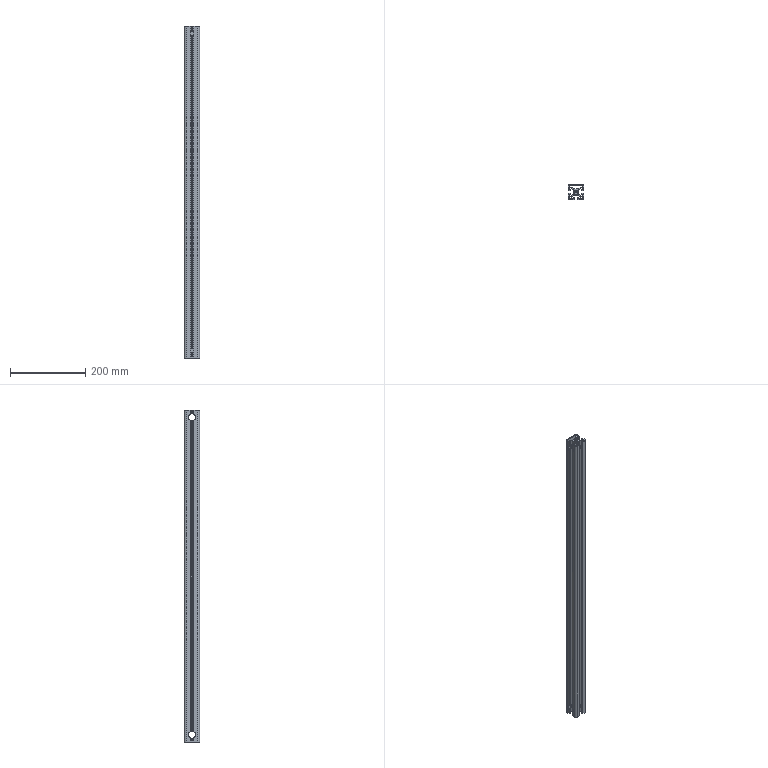Part | SolidWorks | features BaseBody 1, HoleWzd 1, MoveFace 1 | 1 solid | 242 faces | box 40 x 40 x 880 mm | volume 512640 mm3 | plane 187 | cylinder 55 | commonest cylinder face diameters 6.8 x15 2 x14 19 x12 1 x6 5 x4 9 x4